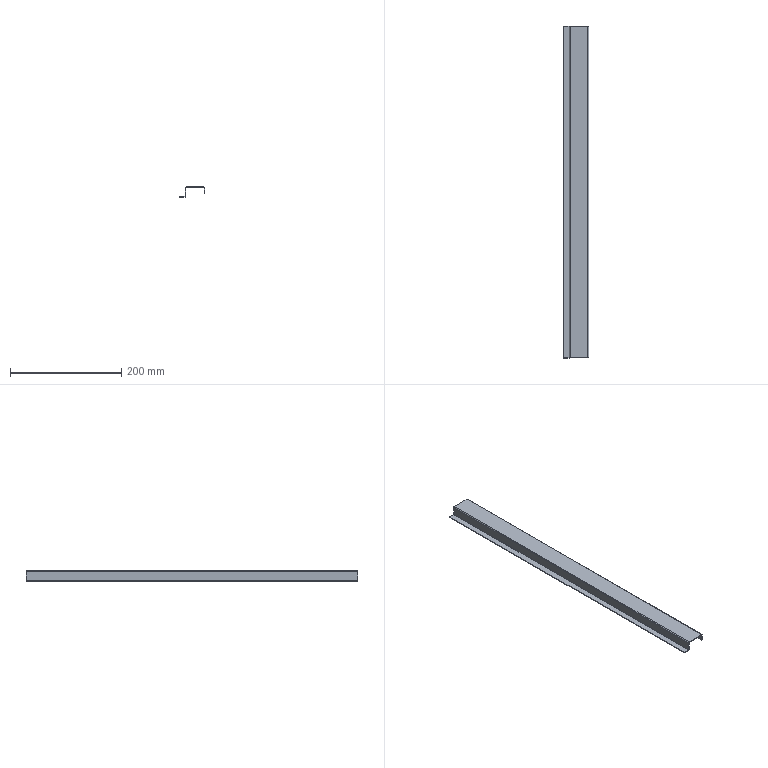Part | SolidWorks | features EdgeFlange 3, FlatPattern 1, SMBaseFlange 1, SheetMetal 1 | 1 solid | 30 faces | box 45.8 x 597 x 18 mm | volume 51846 mm3 | plane 24 | cylinder 6 | commonest cylinder face diameters 0.4 x3 2.8 x3
STEP:
#1=CARTESIAN_POINT('',(0.,0.474,-1.4));
#2=VERTEX_POINT('',#1);
#3=CARTESIAN_POINT('',(0.,0.474,-16.6));
#4=VERTEX_POINT('',#3);
#5=CARTESIAN_POINT('',(0.,0.474,-18.));
#6=DIRECTION('',(0.,0.,-1.));
#7=VECTOR('',#6,1000.);
#8=LINE('',#5,#7);
#9=EDGE_CURVE('',#2,#4,#8,.T.);
#10=ORIENTED_EDGE('',*,*,#9,.T.);
#11=CARTESIAN_POINT('',(1.2,0.474,-16.6));
#12=VERTEX_POINT('',#11);
#13=CARTESIAN_POINT('',(0.,0.474,-16.6));
#14=DIRECTION('',(1.,0.,0.));
#15=VECTOR('',#14,1000.);
#16=LINE('',#13,#15);
#17=EDGE_CURVE('',#4,#12,#16,.T.);
#18=ORIENTED_EDGE('',*,*,#17,.T.);
#19=CARTESIAN_POINT('',(1.2,0.474,-1.4));
#20=VERTEX_POINT('',#19);
#21=CARTESIAN_POINT('',(1.2,0.474,0.));
#22=DIRECTION('',(0.,0.,-1.));
#23=VECTOR('',#22,1000.);
#24=LINE('',#21,#23);
#25=EDGE_CURVE('',#20,#12,#24,.T.);
#26=ORIENTED_EDGE('',*,*,#25,.F.);
#27=CARTESIAN_POINT('',(0.,0.474,-1.4));
#28=DIRECTION('',(-1.,0.,0.));
#29=VECTOR('',#28,1000.);
#30=LINE('',#27,#29);
#31=EDGE_CURVE('',#20,#2,#30,.T.);
#32=ORIENTED_EDGE('',*,*,#31,.T.);
#33=EDGE_LOOP('',(#10,#18,#26,#32));
#34=FACE_OUTER_BOUND('',#33,.T.);
#35=CARTESIAN_POINT('',(0.,0.474,-18.));
#36=DIRECTION('',(0.,-1.,0.));
#37=DIRECTION('',(0.,0.,-1.));
#38=AXIS2_PLACEMENT_3D('',#35,#36,#37);
#39=PLANE('',#38);
#40=ADVANCED_FACE('',(#34),#39,.T.);
#41=CARTESIAN_POINT('',(0.,597.474,-16.6));
#42=VERTEX_POINT('',#41);
#43=CARTESIAN_POINT('',(0.,597.474,-1.4));
#44=VERTEX_POINT('',#43);
#45=CARTESIAN_POINT('',(0.,597.474,-1.2));
#46=DIRECTION('',(0.,0.,1.));
#47=VECTOR('',#46,1000.);
#48=LINE('',#45,#47);
#49=EDGE_CURVE('',#42,#44,#48,.T.);
#50=ORIENTED_EDGE('',*,*,#49,.F.);
#51=CARTESIAN_POINT('',(0.,0.474,-16.6));
#52=DIRECTION('',(0.,1.,0.));
#53=VECTOR('',#52,1000.);
#54=LINE('',#51,#53);
#55=EDGE_CURVE('',#4,#42,#54,.T.);
#56=ORIENTED_EDGE('',*,*,#55,.F.);
#57=ORIENTED_EDGE('',*,*,#9,.F.);
#58=CARTESIAN_POINT('',(0.,0.,-1.4));
#59=DIRECTION('',(0.,1.,0.));
#60=VECTOR('',#59,1000.);
#61=LINE('',#58,#60);
#62=EDGE_CURVE('',#2,#44,#61,.T.);
#63=ORIENTED_EDGE('',*,*,#62,.T.);
#64=EDGE_LOOP('',(#50,#56,#57,#63));
#65=FACE_OUTER_BOUND('',#64,.T.);
#66=CARTESIAN_POINT('',(0.,0.,0.));
#67=DIRECTION('',(-1.,0.,0.));
#68=DIRECTION('',(0.,0.,1.));
#69=AXIS2_PLACEMENT_3D('',#66,#67,#68);
#70=PLANE('',#69);
#71=ADVANCED_FACE('',(#65),#70,.T.);
#72=CARTESIAN_POINT('',(1.2,597.474,-16.6));
#73=VERTEX_POINT('',#72);
#74=CARTESIAN_POINT('',(1.2,0.474,-16.6));
#75=DIRECTION('',(0.,1.,0.));
#76=VECTOR('',#75,1000.);
#77=LINE('',#74,#76);
#78=EDGE_CURVE('',#12,#73,#77,.T.);
#79=ORIENTED_EDGE('',*,*,#78,.T.);
#80=CARTESIAN_POINT('',(1.2,597.474,-1.4));
#81=VERTEX_POINT('',#80);
#82=CARTESIAN_POINT('',(1.2,597.474,0.));
#83=DIRECTION('',(0.,0.,1.));
#84=VECTOR('',#83,1000.);
#85=LINE('',#82,#84);
#86=EDGE_CURVE('',#73,#81,#85,.T.);
#87=ORIENTED_EDGE('',*,*,#86,.T.);
#88=CARTESIAN_POINT('',(1.2,0.474,-1.4));
#89=DIRECTION('',(0.,1.,0.));
#90=VECTOR('',#89,1000.);
#91=LINE('',#88,#90);
#92=EDGE_CURVE('',#20,#81,#91,.T.);
#93=ORIENTED_EDGE('',*,*,#92,.F.);
#94=ORIENTED_EDGE('',*,*,#25,.T.);
#95=EDGE_LOOP('',(#79,#87,#93,#94));
#96=FACE_OUTER_BOUND('',#95,.T.);
#97=CARTESIAN_POINT('',(1.2,0.,0.));
#98=DIRECTION('',(-1.,0.,0.));
#99=DIRECTION('',(0.,0.,1.));
#100=AXIS2_PLACEMENT_3D('',#97,#98,#99);
#101=PLANE('',#100);
#102=ADVANCED_FACE('',(#96),#101,.F.);
#103=CARTESIAN_POINT('',(1.4,0.474,-1.2));
#104=VERTEX_POINT('',#103);
#105=CARTESIAN_POINT('',(33.6,0.474,-1.2));
#106=VERTEX_POINT('',#105);
#107=CARTESIAN_POINT('',(0.,0.474,-1.2));
#108=DIRECTION('',(1.,0.,0.));
#109=VECTOR('',#108,1000.);
#110=LINE('',#107,#109);
#111=EDGE_CURVE('',#104,#106,#110,.T.);
#112=ORIENTED_EDGE('',*,*,#111,.F.);
#113=CARTESIAN_POINT('',(1.4,597.474,-1.2));
#114=VERTEX_POINT('',#113);
#115=CARTESIAN_POINT('',(1.4,597.474,-1.2));
#116=DIRECTION('',(0.,-1.,0.));
#117=VECTOR('',#116,1000.);
#118=LINE('',#115,#117);
#119=EDGE_CURVE('',#114,#104,#118,.T.);
#120=ORIENTED_EDGE('',*,*,#119,.F.);
#121=CARTESIAN_POINT('',(33.6,597.474,-1.2));
#122=VERTEX_POINT('',#121);
#123=CARTESIAN_POINT('',(0.,597.474,-1.2));
#124=DIRECTION('',(-1.,0.,0.));
#125=VECTOR('',#124,1000.);
#126=LINE('',#123,#125);
#127=EDGE_CURVE('',#122,#114,#126,.T.);
#128=ORIENTED_EDGE('',*,*,#127,.F.);
#129=CARTESIAN_POINT('',(33.6,0.474,-1.2));
#130=DIRECTION('',(0.,1.,0.));
#131=VECTOR('',#130,1000.);
#132=LINE('',#129,#131);
#133=EDGE_CURVE('',#106,#122,#132,.T.);
#134=ORIENTED_EDGE('',*,*,#133,.F.);
#135=EDGE_LOOP('',(#112,#120,#128,#134));
#136=FACE_OUTER_BOUND('',#135,.T.);
#137=CARTESIAN_POINT('',(0.,0.,-1.2));
#138=DIRECTION('',(0.,0.,-1.));
#139=DIRECTION('',(-1.,0.,0.));
#140=AXIS2_PLACEMENT_3D('',#137,#138,#139);
#141=PLANE('',#140);
#142=ADVANCED_FACE('',(#136),#141,.T.);
#143=CARTESIAN_POINT('',(1.4,597.474,0.));
#144=VERTEX_POINT('',#143);
#145=CARTESIAN_POINT('',(1.4,0.474,0.));
#146=VERTEX_POINT('',#145);
#147=CARTESIAN_POINT('',(1.4,597.474,0.));
#148=DIRECTION('',(0.,-1.,0.));
#149=VECTOR('',#148,1000.);
#150=LINE('',#147,#149);
#151=EDGE_CURVE('',#144,#146,#150,.T.);
#152=ORIENTED_EDGE('',*,*,#151,.T.);
#153=CARTESIAN_POINT('',(33.6,0.474,0.));
#154=VERTEX_POINT('',#153);
#155=CARTESIAN_POINT('',(0.,0.474,0.));
#156=DIRECTION('',(1.,0.,0.));
#157=VECTOR('',#156,1000.);
#158=LINE('',#155,#157);
#159=EDGE_CURVE('',#146,#154,#158,.T.);
#160=ORIENTED_EDGE('',*,*,#159,.T.);
#161=CARTESIAN_POINT('',(33.6,597.474,0.));
#162=VERTEX_POINT('',#161);
#163=CARTESIAN_POINT('',(33.6,0.474,0.));
#164=DIRECTION('',(0.,1.,0.));
#165=VECTOR('',#164,1000.);
#166=LINE('',#163,#165);
#167=EDGE_CURVE('',#154,#162,#166,.T.);
#168=ORIENTED_EDGE('',*,*,#167,.T.);
#169=CARTESIAN_POINT('',(0.,597.474,0.));
#170=DIRECTION('',(-1.,0.,0.));
#171=VECTOR('',#170,1000.);
#172=LINE('',#169,#171);
#173=EDGE_CURVE('',#162,#144,#172,.T.);
#174=ORIENTED_EDGE('',*,*,#173,.T.);
#175=EDGE_LOOP('',(#152,#160,#168,#174));
#176=FACE_OUTER_BOUND('',#175,.T.);
#177=CARTESIAN_POINT('',(0.,0.,0.));
#178=DIRECTION('',(0.,0.,-1.));
#179=DIRECTION('',(-1.,0.,0.));
#180=AXIS2_PLACEMENT_3D('',#177,#178,#179);
#181=PLANE('',#180);
#182=ADVANCED_FACE('',(#176),#181,.F.);
#183=ORIENTED_EDGE('',*,*,#127,.T.);
#184=CARTESIAN_POINT('',(1.4,597.474,-1.2));
#185=DIRECTION('',(0.,0.,1.));
#186=VECTOR('',#185,1000.);
#187=LINE('',#184,#186);
#188=EDGE_CURVE('',#114,#144,#187,.T.);
#189=ORIENTED_EDGE('',*,*,#188,.T.);
#190=ORIENTED_EDGE('',*,*,#173,.F.);
#191=CARTESIAN_POINT('',(33.6,597.474,-1.2));
#192=DIRECTION('',(0.,0.,1.));
#193=VECTOR('',#192,1000.);
#194=LINE('',#191,#193);
#195=EDGE_CURVE('',#122,#162,#194,.T.);
#196=ORIENTED_EDGE('',*,*,#195,.F.);
#197=EDGE_LOOP('',(#183,#189,#190,#196));
#198=FACE_OUTER_BOUND('',#197,.T.);
#199=CARTESIAN_POINT('',(0.,597.474,-1.2));
#200=DIRECTION('',(0.,1.,0.));
#201=DIRECTION('',(0.,0.,1.));
#202=AXIS2_PLACEMENT_3D('',#199,#200,#201);
#203=PLANE('',#202);
#204=ADVANCED_FACE('',(#198),#203,.T.);
#205=CARTESIAN_POINT('',(1.4,0.474,-1.2));
#206=DIRECTION('',(0.,0.,1.));
#207=VECTOR('',#206,1000.);
#208=LINE('',#205,#207);
#209=EDGE_CURVE('',#104,#146,#208,.T.);
#210=ORIENTED_EDGE('',*,*,#209,.F.);
#211=ORIENTED_EDGE('',*,*,#111,.T.);
#212=CARTESIAN_POINT('',(33.6,0.474,-1.2));
#213=DIRECTION('',(0.,0.,1.));
#214=VECTOR('',#213,1000.);
#215=LINE('',#212,#214);
#216=EDGE_CURVE('',#106,#154,#215,.T.);
#217=ORIENTED_EDGE('',*,*,#216,.T.);
#218=ORIENTED_EDGE('',*,*,#159,.F.);
#219=EDGE_LOOP('',(#210,#211,#217,#218));
#220=FACE_OUTER_BOUND('',#219,.T.);
#221=CARTESIAN_POINT('',(0.,0.474,-1.2));
#222=DIRECTION('',(0.,-1.,0.));
#223=DIRECTION('',(0.,0.,-1.));
#224=AXIS2_PLACEMENT_3D('',#221,#222,#223);
#225=PLANE('',#224);
#226=ADVANCED_FACE('',(#220),#225,.T.);
#227=CARTESIAN_POINT('',(33.8,597.474,-1.4));
#228=VERTEX_POINT('',#227);
#229=CARTESIAN_POINT('',(35.,597.474,-1.4));
#230=VERTEX_POINT('',#229);
#231=CARTESIAN_POINT('',(35.,597.474,-1.4));
#232=DIRECTION('',(1.,0.,0.));
#233=VECTOR('',#232,1000.);
#234=LINE('',#231,#233);
#235=EDGE_CURVE('',#228,#230,#234,.T.);
#236=ORIENTED_EDGE('',*,*,#235,.F.);
#237=CARTESIAN_POINT('',(33.6,597.474,-1.4));
#238=DIRECTION('',(0.,1.,0.));
#239=DIRECTION('',(0.,0.,-1.));
#240=AXIS2_PLACEMENT_3D('',#237,#238,#239);
#241=CIRCLE('',#240,0.2);
#242=EDGE_CURVE('',#122,#228,#241,.T.);
#243=ORIENTED_EDGE('',*,*,#242,.F.);
#244=ORIENTED_EDGE('',*,*,#195,.T.);
#245=CARTESIAN_POINT('',(33.6,597.474,-1.4));
#246=DIRECTION('',(0.,1.,0.));
#247=DIRECTION('',(0.,0.,-1.));
#248=AXIS2_PLACEMENT_3D('',#245,#246,#247);
#249=CIRCLE('',#248,1.4);
#250=EDGE_CURVE('',#162,#230,#249,.T.);
#251=ORIENTED_EDGE('',*,*,#250,.T.);
#252=EDGE_LOOP('',(#236,#243,#244,#251));
#253=FACE_OUTER_BOUND('',#252,.T.);
#254=CARTESIAN_POINT('',(33.6,597.474,-1.4));
#255=DIRECTION('',(0.,1.,0.));
#256=DIRECTION('',(0.,0.,1.));
#257=AXIS2_PLACEMENT_3D('',#254,#255,#256);
#258=PLANE('',#257);
#259=ADVANCED_FACE('',(#253),#258,.T.);
#260=CARTESIAN_POINT('',(33.8,0.474,-1.4));
#261=VERTEX_POINT('',#260);
#262=CARTESIAN_POINT('',(33.6,0.474,-1.4));
#263=DIRECTION('',(0.,-1.,0.));
#264=DIRECTION('',(0.,0.,-1.));
#265=AXIS2_PLACEMENT_3D('',#262,#263,#264);
#266=CIRCLE('',#265,0.2);
#267=EDGE_CURVE('',#261,#106,#266,.T.);
#268=ORIENTED_EDGE('',*,*,#267,.F.);
#269=CARTESIAN_POINT('',(35.,0.474,-1.4));
#270=VERTEX_POINT('',#269);
#271=CARTESIAN_POINT('',(33.8,0.474,-1.4));
#272=DIRECTION('',(1.,0.,0.));
#273=VECTOR('',#272,1000.);
#274=LINE('',#271,#273);
#275=EDGE_CURVE('',#261,#270,#274,.T.);
#276=ORIENTED_EDGE('',*,*,#275,.T.);
#277=CARTESIAN_POINT('',(33.6,0.474,-1.4));
#278=DIRECTION('',(0.,-1.,0.));
#279=DIRECTION('',(0.,0.,-1.));
#280=AXIS2_PLACEMENT_3D('',#277,#278,#279);
#281=CIRCLE('',#280,1.4);
#282=EDGE_CURVE('',#270,#154,#281,.T.);
#283=ORIENTED_EDGE('',*,*,#282,.T.);
#284=ORIENTED_EDGE('',*,*,#216,.F.);
#285=EDGE_LOOP('',(#268,#276,#283,#284));
#286=FACE_OUTER_BOUND('',#285,.T.);
#287=CARTESIAN_POINT('',(33.6,0.474,-1.4));
#288=DIRECTION('',(0.,1.,0.));
#289=DIRECTION('',(0.,0.,1.));
#290=AXIS2_PLACEMENT_3D('',#287,#288,#289);
#291=PLANE('',#290);
#292=ADVANCED_FACE('',(#286),#291,.F.);
#293=ORIENTED_EDGE('',*,*,#167,.F.);
#294=ORIENTED_EDGE('',*,*,#282,.F.);
#295=CARTESIAN_POINT('',(35.,0.,-1.4));
#296=DIRECTION('',(0.,-1.,0.));
#297=VECTOR('',#296,1000.);
#298=LINE('',#295,#297);
#299=EDGE_CURVE('',#230,#270,#298,.T.);
#300=ORIENTED_EDGE('',*,*,#299,.F.);
#301=ORIENTED_EDGE('',*,*,#250,.F.);
#302=EDGE_LOOP('',(#293,#294,#300,#301));
#303=FACE_OUTER_BOUND('',#302,.T.);
#304=CARTESIAN_POINT('',(33.6,0.474,-1.4));
#305=DIRECTION('',(0.,-1.,0.));
#306=DIRECTION('',(1.,0.,0.));
#307=AXIS2_PLACEMENT_3D('',#304,#305,#306);
#308=CYLINDRICAL_SURFACE('',#307,1.4);
#309=ADVANCED_FACE('',(#303),#308,.T.);
#310=ORIENTED_EDGE('',*,*,#133,.T.);
#311=ORIENTED_EDGE('',*,*,#242,.T.);
#312=CARTESIAN_POINT('',(33.8,597.474,-1.4));
#313=DIRECTION('',(0.,-1.,0.));
#314=VECTOR('',#313,1000.);
#315=LINE('',#312,#314);
#316=EDGE_CURVE('',#228,#261,#315,.T.);
#317=ORIENTED_EDGE('',*,*,#316,.T.);
#318=ORIENTED_EDGE('',*,*,#267,.T.);
#319=EDGE_LOOP('',(#310,#311,#317,#318));
#320=FACE_OUTER_BOUND('',#319,.T.);
#321=CARTESIAN_POINT('',(33.6,0.474,-1.4));
#322=DIRECTION('',(0.,-1.,0.));
#323=DIRECTION('',(1.,0.,0.));
#324=AXIS2_PLACEMENT_3D('',#321,#322,#323);
#325=CYLINDRICAL_SURFACE('',#324,0.2);
#326=ADVANCED_FACE('',(#320),#325,.F.);
#327=CARTESIAN_POINT('',(35.,0.474,-12.));
#328=VERTEX_POINT('',#327);
#329=CARTESIAN_POINT('',(35.,0.474,-1.2));
#330=DIRECTION('',(0.,0.,1.));
#331=VECTOR('',#330,1000.);
#332=LINE('',#329,#331);
#333=EDGE_CURVE('',#328,#270,#332,.T.);
#334=ORIENTED_EDGE('',*,*,#333,.T.);
#335=ORIENTED_EDGE('',*,*,#275,.F.);
#336=CARTESIAN_POINT('',(33.8,0.474,-12.));
#337=VERTEX_POINT('',#336);
#338=CARTESIAN_POINT('',(33.8,0.474,0.));
#339=DIRECTION('',(0.,0.,1.));
#340=VECTOR('',#339,1000.);
#341=LINE('',#338,#340);
#342=EDGE_CURVE('',#337,#261,#341,.T.);
#343=ORIENTED_EDGE('',*,*,#342,.F.);
#344=CARTESIAN_POINT('',(35.,0.474,-12.));
#345=DIRECTION('',(-1.,0.,0.));
#346=VECTOR('',#345,1000.);
#347=LINE('',#344,#346);
#348=EDGE_CURVE('',#328,#337,#347,.T.);
#349=ORIENTED_EDGE('',*,*,#348,.F.);
#350=EDGE_LOOP('',(#334,#335,#343,#349));
#351=FACE_OUTER_BOUND('',#350,.T.);
#352=CARTESIAN_POINT('',(35.,0.474,-1.2));
#353=DIRECTION('',(0.,-1.,0.));
#354=DIRECTION('',(0.,0.,-1.));
#355=AXIS2_PLACEMENT_3D('',#352,#353,#354);
#356=PLANE('',#355);
#357=ADVANCED_FACE('',(#351),#356,.T.);
#358=CARTESIAN_POINT('',(33.8,597.474,-12.));
#359=VERTEX_POINT('',#358);
#360=CARTESIAN_POINT('',(33.8,597.474,0.));
#361=DIRECTION('',(0.,0.,-1.));
#362=VECTOR('',#361,1000.);
#363=LINE('',#360,#362);
#364=EDGE_CURVE('',#228,#359,#363,.T.);
#365=ORIENTED_EDGE('',*,*,#364,.F.);
#366=ORIENTED_EDGE('',*,*,#235,.T.);
#367=CARTESIAN_POINT('',(35.,597.474,-12.));
#368=VERTEX_POINT('',#367);
#369=CARTESIAN_POINT('',(35.,597.474,-12.));
#370=DIRECTION('',(0.,0.,-1.));
#371=VECTOR('',#370,1000.);
#372=LINE('',#369,#371);
#373=EDGE_CURVE('',#230,#368,#372,.T.);
#374=ORIENTED_EDGE('',*,*,#373,.T.);
#375=CARTESIAN_POINT('',(35.,597.474,-12.));
#376=DIRECTION('',(-1.,0.,0.));
#377=VECTOR('',#376,1000.);
#378=LINE('',#375,#377);
#379=EDGE_CURVE('',#368,#359,#378,.T.);
#380=ORIENTED_EDGE('',*,*,#379,.T.);
#381=EDGE_LOOP('',(#365,#366,#374,#380));
#382=FACE_OUTER_BOUND('',#381,.T.);
#383=CARTESIAN_POINT('',(35.,597.474,-12.));
#384=DIRECTION('',(0.,1.,0.));
#385=DIRECTION('',(0.,0.,1.));
#386=AXIS2_PLACEMENT_3D('',#383,#384,#385);
#387=PLANE('',#386);
#388=ADVANCED_FACE('',(#382),#387,.T.);
#389=ORIENTED_EDGE('',*,*,#373,.F.);
#390=ORIENTED_EDGE('',*,*,#299,.T.);
#391=ORIENTED_EDGE('',*,*,#333,.F.);
#392=CARTESIAN_POINT('',(35.,0.474,-12.));
#393=DIRECTION('',(0.,-1.,0.));
#394=VECTOR('',#393,1000.);
#395=LINE('',#392,#394);
#396=EDGE_CURVE('',#368,#328,#395,.T.);
#397=ORIENTED_EDGE('',*,*,#396,.F.);
#398=EDGE_LOOP('',(#389,#390,#391,#397));
#399=FACE_OUTER_BOUND('',#398,.T.);
#400=CARTESIAN_POINT('',(35.,0.,0.));
#401=DIRECTION('',(1.,0.,0.));
#402=DIRECTION('',(0.,0.,-1.));
#403=AXIS2_PLACEMENT_3D('',#400,#401,#402);
#404=PLANE('',#403);
#405=ADVANCED_FACE('',(#399),#404,.T.);
#406=ORIENTED_EDGE('',*,*,#316,.F.);
#407=ORIENTED_EDGE('',*,*,#364,.T.);
#408=CARTESIAN_POINT('',(33.8,0.,-12.));
#409=DIRECTION('',(0.,-1.,0.));
#410=VECTOR('',#409,1000.);
#411=LINE('',#408,#410);
#412=EDGE_CURVE('',#359,#337,#411,.T.);
#413=ORIENTED_EDGE('',*,*,#412,.T.);
#414=ORIENTED_EDGE('',*,*,#342,.T.);
#415=EDGE_LOOP('',(#406,#407,#413,#414));
#416=FACE_OUTER_BOUND('',#415,.T.);
#417=CARTESIAN_POINT('',(33.8,0.,0.));
#418=DIRECTION('',(1.,0.,0.));
#419=DIRECTION('',(0.,0.,-1.));
#420=AXIS2_PLACEMENT_3D('',#417,#418,#419);
#421=PLANE('',#420);
#422=ADVANCED_FACE('',(#416),#421,.F.);
#423=ORIENTED_EDGE('',*,*,#412,.F.);
#424=ORIENTED_EDGE('',*,*,#379,.F.);
#425=ORIENTED_EDGE('',*,*,#396,.T.);
#426=ORIENTED_EDGE('',*,*,#348,.T.);
#427=EDGE_LOOP('',(#423,#424,#425,#426));
#428=FACE_OUTER_BOUND('',#427,.T.);
#429=CARTESIAN_POINT('',(35.,0.474,-12.));
#430=DIRECTION('',(0.,0.,-1.));
#431=DIRECTION('',(-1.,0.,0.));
#432=AXIS2_PLACEMENT_3D('',#429,#430,#431);
#433=PLANE('',#432);
#434=ADVANCED_FACE('',(#428),#433,.T.);
#435=ORIENTED_EDGE('',*,*,#31,.F.);
#436=CARTESIAN_POINT('',(1.4,0.474,-1.4));
#437=DIRECTION('',(0.,-1.,0.));
#438=DIRECTION('',(0.,0.,1.));
#439=AXIS2_PLACEMENT_3D('',#436,#437,#438);
#440=CIRCLE('',#439,0.2);
#441=EDGE_CURVE('',#104,#20,#440,.T.);
#442=ORIENTED_EDGE('',*,*,#441,.F.);
#443=ORIENTED_EDGE('',*,*,#209,.T.);
#444=CARTESIAN_POINT('',(1.4,0.474,-1.4));
#445=DIRECTION('',(0.,-1.,0.));
#446=DIRECTION('',(0.,0.,1.));
#447=AXIS2_PLACEMENT_3D('',#444,#445,#446);
#448=CIRCLE('',#447,1.4);
#449=EDGE_CURVE('',#146,#2,#448,.T.);
#450=ORIENTED_EDGE('',*,*,#449,.T.);
#451=EDGE_LOOP('',(#435,#442,#443,#450));
#452=FACE_OUTER_BOUND('',#451,.T.);
#453=CARTESIAN_POINT('',(1.4,0.474,-1.4));
#454=DIRECTION('',(0.,-1.,0.));
#455=DIRECTION('',(0.,0.,-1.));
#456=AXIS2_PLACEMENT_3D('',#453,#454,#455);
#457=PLANE('',#456);
#458=ADVANCED_FACE('',(#452),#457,.T.);
#459=CARTESIAN_POINT('',(1.4,597.474,-1.4));
#460=DIRECTION('',(0.,1.,0.));
#461=DIRECTION('',(0.,0.,1.));
#462=AXIS2_PLACEMENT_3D('',#459,#460,#461);
#463=CIRCLE('',#462,0.2);
#464=EDGE_CURVE('',#81,#114,#463,.T.);
#465=ORIENTED_EDGE('',*,*,#464,.F.);
#466=CARTESIAN_POINT('',(1.2,597.474,-1.4));
#467=DIRECTION('',(-1.,0.,0.));
#468=VECTOR('',#467,1000.);
#469=LINE('',#466,#468);
#470=EDGE_CURVE('',#81,#44,#469,.T.);
#471=ORIENTED_EDGE('',*,*,#470,.T.);
#472=CARTESIAN_POINT('',(1.4,597.474,-1.4));
#473=DIRECTION('',(0.,1.,0.));
#474=DIRECTION('',(0.,0.,1.));
#475=AXIS2_PLACEMENT_3D('',#472,#473,#474);
#476=CIRCLE('',#475,1.4);
#477=EDGE_CURVE('',#44,#144,#476,.T.);
#478=ORIENTED_EDGE('',*,*,#477,.T.);
#479=ORIENTED_EDGE('',*,*,#188,.F.);
#480=EDGE_LOOP('',(#465,#471,#478,#479));
#481=FACE_OUTER_BOUND('',#480,.T.);
#482=CARTESIAN_POINT('',(1.4,597.474,-1.4));
#483=DIRECTION('',(0.,-1.,0.));
#484=DIRECTION('',(0.,0.,-1.));
#485=AXIS2_PLACEMENT_3D('',#482,#483,#484);
#486=PLANE('',#485);
#487=ADVANCED_FACE('',(#481),#486,.F.);
#488=ORIENTED_EDGE('',*,*,#151,.F.);
#489=ORIENTED_EDGE('',*,*,#477,.F.);
#490=ORIENTED_EDGE('',*,*,#62,.F.);
#491=ORIENTED_EDGE('',*,*,#449,.F.);
#492=EDGE_LOOP('',(#488,#489,#490,#491));
#493=FACE_OUTER_BOUND('',#492,.T.);
#494=CARTESIAN_POINT('',(1.4,597.474,-1.4));
#495=DIRECTION('',(0.,1.,0.));
#496=DIRECTION('',(-1.,0.,0.));
#497=AXIS2_PLACEMENT_3D('',#494,#495,#496);
#498=CYLINDRICAL_SURFACE('',#497,1.4);
#499=ADVANCED_FACE('',(#493),#498,.T.);
#500=ORIENTED_EDGE('',*,*,#119,.T.);
#501=ORIENTED_EDGE('',*,*,#441,.T.);
#502=ORIENTED_EDGE('',*,*,#92,.T.);
#503=ORIENTED_EDGE('',*,*,#464,.T.);
#504=EDGE_LOOP('',(#500,#501,#502,#503));
#505=FACE_OUTER_BOUND('',#504,.T.);
#506=CARTESIAN_POINT('',(1.4,597.474,-1.4));
#507=DIRECTION('',(0.,1.,0.));
#508=DIRECTION('',(-1.,0.,0.));
#509=AXIS2_PLACEMENT_3D('',#506,#507,#508);
#510=CYLINDRICAL_SURFACE('',#509,0.2);
#511=ADVANCED_FACE('',(#505),#510,.F.);
#512=CARTESIAN_POINT('',(0.,597.474,-16.6));
#513=DIRECTION('',(1.,0.,0.));
#514=VECTOR('',#513,1000.);
#515=LINE('',#512,#514);
#516=EDGE_CURVE('',#42,#73,#515,.T.);
#517=ORIENTED_EDGE('',*,*,#516,.F.);
#518=ORIENTED_EDGE('',*,*,#49,.T.);
#519=ORIENTED_EDGE('',*,*,#470,.F.);
#520=ORIENTED_EDGE('',*,*,#86,.F.);
#521=EDGE_LOOP('',(#517,#518,#519,#520));
#522=FACE_OUTER_BOUND('',#521,.T.);
#523=CARTESIAN_POINT('',(0.,597.474,-1.2));
#524=DIRECTION('',(0.,1.,0.));
#525=DIRECTION('',(0.,0.,1.));
#526=AXIS2_PLACEMENT_3D('',#523,#524,#525);
#527=PLANE('',#526);
#528=ADVANCED_FACE('',(#522),#527,.T.);
#529=CARTESIAN_POINT('',(-0.2,597.474,-16.8));
#530=VERTEX_POINT('',#529);
#531=CARTESIAN_POINT('',(-0.2,597.474,-18.));
#532=VERTEX_POINT('',#531);
#533=CARTESIAN_POINT('',(-0.2,597.474,-18.));
#534=DIRECTION('',(0.,0.,-1.));
#535=VECTOR('',#534,1000.);
#536=LINE('',#533,#535);
#537=EDGE_CURVE('',#530,#532,#536,.T.);
#538=ORIENTED_EDGE('',*,*,#537,.F.);
#539=CARTESIAN_POINT('',(-0.2,597.474,-16.6));
#540=DIRECTION('',(0.,1.,0.));
#541=DIRECTION('',(0.,0.,-1.));
#542=AXIS2_PLACEMENT_3D('',#539,#540,#541);
#543=CIRCLE('',#542,0.2);
#544=EDGE_CURVE('',#42,#530,#543,.T.);
#545=ORIENTED_EDGE('',*,*,#544,.F.);
#546=ORIENTED_EDGE('',*,*,#516,.T.);
#547=CARTESIAN_POINT('',(-0.2,597.474,-16.6));
#548=DIRECTION('',(0.,1.,0.));
#549=DIRECTION('',(0.,0.,-1.));
#550=AXIS2_PLACEMENT_3D('',#547,#548,#549);
#551=CIRCLE('',#550,1.4);
#552=EDGE_CURVE('',#73,#532,#551,.T.);
#553=ORIENTED_EDGE('',*,*,#552,.T.);
#554=EDGE_LOOP('',(#538,#545,#546,#553));
#555=FACE_OUTER_BOUND('',#554,.T.);
#556=CARTESIAN_POINT('',(-0.2,597.474,-16.6));
#557=DIRECTION('',(0.,1.,0.));
#558=DIRECTION('',(0.,0.,1.));
#559=AXIS2_PLACEMENT_3D('',#556,#557,#558);
#560=PLANE('',#559);
#561=ADVANCED_FACE('',(#555),#560,.T.);
#562=CARTESIAN_POINT('',(-0.2,0.474,-16.8));
#563=VERTEX_POINT('',#562);
#564=CARTESIAN_POINT('',(-0.2,0.474,-16.6));
#565=DIRECTION('',(0.,-1.,0.));
#566=DIRECTION('',(0.,0.,-1.));
#567=AXIS2_PLACEMENT_3D('',#564,#565,#566);
#568=CIRCLE('',#567,0.2);
#569=EDGE_CURVE('',#563,#4,#568,.T.);
#570=ORIENTED_EDGE('',*,*,#569,.F.);
#571=CARTESIAN_POINT('',(-0.2,0.474,-18.));
#572=VERTEX_POINT('',#571);
#573=CARTESIAN_POINT('',(-0.2,0.474,-16.8));
#574=DIRECTION('',(0.,0.,-1.));
#575=VECTOR('',#574,1000.);
#576=LINE('',#573,#575);
#577=EDGE_CURVE('',#563,#572,#576,.T.);
#578=ORIENTED_EDGE('',*,*,#577,.T.);
#579=CARTESIAN_POINT('',(-0.2,0.474,-16.6));
#580=DIRECTION('',(0.,-1.,0.));
#581=DIRECTION('',(0.,0.,-1.));
#582=AXIS2_PLACEMENT_3D('',#579,#580,#581);
#583=CIRCLE('',#582,1.4);
#584=EDGE_CURVE('',#572,#12,#583,.T.);
#585=ORIENTED_EDGE('',*,*,#584,.T.);
#586=ORIENTED_EDGE('',*,*,#17,.F.);
#587=EDGE_LOOP('',(#570,#578,#585,#586));
#588=FACE_OUTER_BOUND('',#587,.T.);
#589=CARTESIAN_POINT('',(-0.2,0.474,-16.6));
#590=DIRECTION('',(0.,1.,0.));
#591=DIRECTION('',(0.,0.,1.));
#592=AXIS2_PLACEMENT_3D('',#589,#590,#591);
#593=PLANE('',#592);
#594=ADVANCED_FACE('',(#588),#593,.F.);
#595=ORIENTED_EDGE('',*,*,#78,.F.);
#596=ORIENTED_EDGE('',*,*,#584,.F.);
#597=CARTESIAN_POINT('',(-0.2,0.,-18.));
#598=DIRECTION('',(0.,-1.,0.));
#599=VECTOR('',#598,1000.);
#600=LINE('',#597,#599);
#601=EDGE_CURVE('',#532,#572,#600,.T.);
#602=ORIENTED_EDGE('',*,*,#601,.F.);
#603=ORIENTED_EDGE('',*,*,#552,.F.);
#604=EDGE_LOOP('',(#595,#596,#602,#603));
#605=FACE_OUTER_BOUND('',#604,.T.);
#606=CARTESIAN_POINT('',(-0.2,0.474,-16.6));
#607=DIRECTION('',(0.,-1.,0.));
#608=DIRECTION('',(0.,0.,-1.));
#609=AXIS2_PLACEMENT_3D('',#606,#607,#608);
#610=CYLINDRICAL_SURFACE('',#609,1.4);
#611=ADVANCED_FACE('',(#605),#610,.T.);
#612=ORIENTED_EDGE('',*,*,#55,.T.);
#613=ORIENTED_EDGE('',*,*,#544,.T.);
#614=CARTESIAN_POINT('',(-0.2,597.474,-16.8));
#615=DIRECTION('',(0.,-1.,0.));
#616=VECTOR('',#615,1000.);
#617=LINE('',#614,#616);
#618=EDGE_CURVE('',#530,#563,#617,.T.);
#619=ORIENTED_EDGE('',*,*,#618,.T.);
#620=ORIENTED_EDGE('',*,*,#569,.T.);
#621=EDGE_LOOP('',(#612,#613,#619,#620));
#622=FACE_OUTER_BOUND('',#621,.T.);
#623=CARTESIAN_POINT('',(-0.2,0.474,-16.6));
#624=DIRECTION('',(0.,-1.,0.));
#625=DIRECTION('',(0.,0.,-1.));
#626=AXIS2_PLACEMENT_3D('',#623,#624,#625);
#627=CYLINDRICAL_SURFACE('',#626,0.2);
#628=ADVANCED_FACE('',(#622),#627,.F.);
#629=CARTESIAN_POINT('',(-10.8,0.474,-18.));
#630=VERTEX_POINT('',#629);
#631=CARTESIAN_POINT('',(0.,0.474,-18.));
#632=DIRECTION('',(1.,0.,0.));
#633=VECTOR('',#632,1000.);
#634=LINE('',#631,#633);
#635=EDGE_CURVE('',#630,#572,#634,.T.);
#636=ORIENTED_EDGE('',*,*,#635,.T.);
#637=ORIENTED_EDGE('',*,*,#577,.F.);
#638=CARTESIAN_POINT('',(-10.8,0.474,-16.8));
#639=VERTEX_POINT('',#638);
#640=CARTESIAN_POINT('',(0.,0.474,-16.8));
#641=DIRECTION('',(1.,0.,0.));
#642=VECTOR('',#641,1000.);
#643=LINE('',#640,#642);
#644=EDGE_CURVE('',#639,#563,#643,.T.);
#645=ORIENTED_EDGE('',*,*,#644,.F.);
#646=CARTESIAN_POINT('',(-10.8,0.474,-18.));
#647=DIRECTION('',(0.,0.,1.));
#648=VECTOR('',#647,1000.);
#649=LINE('',#646,#648);
#650=EDGE_CURVE('',#630,#639,#649,.T.);
#651=ORIENTED_EDGE('',*,*,#650,.F.);
#652=EDGE_LOOP('',(#636,#637,#645,#651));
#653=FACE_OUTER_BOUND('',#652,.T.);
#654=CARTESIAN_POINT('',(0.,0.474,-18.));
#655=DIRECTION('',(0.,-1.,0.));
#656=DIRECTION('',(1.,0.,0.));
#657=AXIS2_PLACEMENT_3D('',#654,#655,#656);
#658=PLANE('',#657);
#659=ADVANCED_FACE('',(#653),#658,.T.);
#660=CARTESIAN_POINT('',(-10.8,597.474,-16.8));
#661=VERTEX_POINT('',#660);
#662=CARTESIAN_POINT('',(0.,597.474,-16.8));
#663=DIRECTION('',(-1.,0.,0.));
#664=VECTOR('',#663,1000.);
#665=LINE('',#662,#664);
#666=EDGE_CURVE('',#530,#661,#665,.T.);
#667=ORIENTED_EDGE('',*,*,#666,.F.);
#668=ORIENTED_EDGE('',*,*,#537,.T.);
#669=CARTESIAN_POINT('',(-10.8,597.474,-18.));
#670=VERTEX_POINT('',#669);
#671=CARTESIAN_POINT('',(-10.8,597.474,-18.));
#672=DIRECTION('',(-1.,0.,0.));
#673=VECTOR('',#672,1000.);
#674=LINE('',#671,#673);
#675=EDGE_CURVE('',#532,#670,#674,.T.);
#676=ORIENTED_EDGE('',*,*,#675,.T.);
#677=CARTESIAN_POINT('',(-10.8,597.474,-18.));
#678=DIRECTION('',(0.,0.,1.));
#679=VECTOR('',#678,1000.);
#680=LINE('',#677,#679);
#681=EDGE_CURVE('',#670,#661,#680,.T.);
#682=ORIENTED_EDGE('',*,*,#681,.T.);
#683=EDGE_LOOP('',(#667,#668,#676,#682));
#684=FACE_OUTER_BOUND('',#683,.T.);
#685=CARTESIAN_POINT('',(-10.8,597.474,-18.));
#686=DIRECTION('',(0.,1.,0.));
#687=DIRECTION('',(0.,0.,1.));
#688=AXIS2_PLACEMENT_3D('',#685,#686,#687);
#689=PLANE('',#688);
#690=ADVANCED_FACE('',(#684),#689,.T.);
#691=ORIENTED_EDGE('',*,*,#675,.F.);
#692=ORIENTED_EDGE('',*,*,#601,.T.);
#693=ORIENTED_EDGE('',*,*,#635,.F.);
#694=CARTESIAN_POINT('',(-10.8,0.474,-18.));
#695=DIRECTION('',(0.,-1.,0.));
#696=VECTOR('',#695,1000.);
#697=LINE('',#694,#696);
#698=EDGE_CURVE('',#670,#630,#697,.T.);
#699=ORIENTED_EDGE('',*,*,#698,.F.);
#700=EDGE_LOOP('',(#691,#692,#693,#699));
#701=FACE_OUTER_BOUND('',#700,.T.);
#702=CARTESIAN_POINT('',(0.,0.,-18.));
#703=DIRECTION('',(0.,0.,-1.));
#704=DIRECTION('',(-1.,0.,0.));
#705=AXIS2_PLACEMENT_3D('',#702,#703,#704);
#706=PLANE('',#705);
#707=ADVANCED_FACE('',(#701),#706,.T.);
#708=ORIENTED_EDGE('',*,*,#618,.F.);
#709=ORIENTED_EDGE('',*,*,#666,.T.);
#710=CARTESIAN_POINT('',(-10.8,0.,-16.8));
#711=DIRECTION('',(0.,-1.,0.));
#712=VECTOR('',#711,1000.);
#713=LINE('',#710,#712);
#714=EDGE_CURVE('',#661,#639,#713,.T.);
#715=ORIENTED_EDGE('',*,*,#714,.T.);
#716=ORIENTED_EDGE('',*,*,#644,.T.);
#717=EDGE_LOOP('',(#708,#709,#715,#716));
#718=FACE_OUTER_BOUND('',#717,.T.);
#719=CARTESIAN_POINT('',(0.,0.,-16.8));
#720=DIRECTION('',(0.,0.,-1.));
#721=DIRECTION('',(-1.,0.,0.));
#722=AXIS2_PLACEMENT_3D('',#719,#720,#721);
#723=PLANE('',#722);
#724=ADVANCED_FACE('',(#718),#723,.F.);
#725=ORIENTED_EDGE('',*,*,#714,.F.);
#726=ORIENTED_EDGE('',*,*,#681,.F.);
#727=ORIENTED_EDGE('',*,*,#698,.T.);
#728=ORIENTED_EDGE('',*,*,#650,.T.);
#729=EDGE_LOOP('',(#725,#726,#727,#728));
#730=FACE_OUTER_BOUND('',#729,.T.);
#731=CARTESIAN_POINT('',(-10.8,0.474,-18.));
#732=DIRECTION('',(-1.,0.,0.));
#733=DIRECTION('',(0.,0.,1.));
#734=AXIS2_PLACEMENT_3D('',#731,#732,#733);
#735=PLANE('',#734);
#736=ADVANCED_FACE('',(#730),#735,.T.);
#737=CLOSED_SHELL('',(#40,#71,#102,#142,#182,#204,#226,#259,#292,#309,#326,#357,#388,#405,#422,#434,#458,#487,#499,#511,#528,#561,#594,#611,#628,#659,#690,#707,#724,#736));
#738=MANIFOLD_SOLID_BREP('',#737);
#739=CARTESIAN_POINT('',(0.,0.,0.));
#740=DIRECTION('',(0.,0.,1.));
#741=DIRECTION('',(1.,0.,0.));
#742=AXIS2_PLACEMENT_3D('',#739,#740,#741);
#743=(LENGTH_UNIT()NAMED_UNIT(*)SI_UNIT(.MILLI.,.METRE.));
#744=UNCERTAINTY_MEASURE_WITH_UNIT(LENGTH_MEASURE(0.00001),#743,'','');
#745=(NAMED_UNIT(*)PLANE_ANGLE_UNIT()SI_UNIT($,.RADIAN.));
#746=(NAMED_UNIT(*)SI_UNIT($,.STERADIAN.)SOLID_ANGLE_UNIT());
#747=(GEOMETRIC_REPRESENTATION_CONTEXT(3)GLOBAL_UNCERTAINTY_ASSIGNED_CONTEXT((#744))GLOBAL_UNIT_ASSIGNED_CONTEXT((#743,#745,#746))REPRESENTATION_CONTEXT('',''));
#748=ADVANCED_BREP_SHAPE_REPRESENTATION('',(#738,#742),#747);